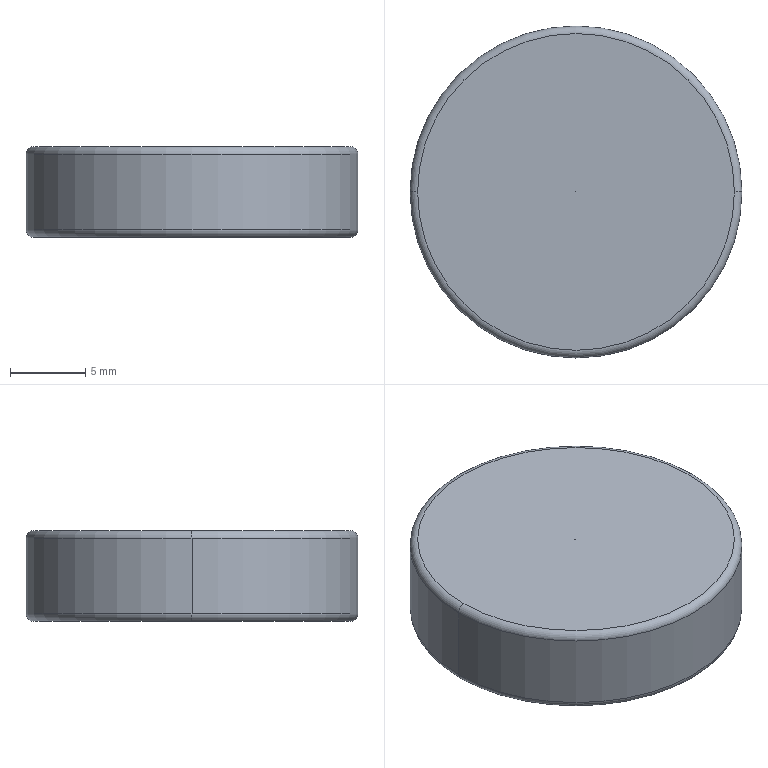Part | STEP file | H_ND24021-01-JG-036-SL | 1 solid | 12 faces | box 22 x 22 x 6 mm | volume 2228 mm3 | torus 4 | cylinder 4 | cone 2 | plane 2 | commonest cylinder face diameters 3.3 x2 22 x2
STEP:
#1=CARTESIAN_POINT('',(0.,0.,0.));
#2=DIRECTION('',(0.,0.,1.));
#3=DIRECTION('',(1.,0.,0.));
#4=AXIS2_PLACEMENT_3D('',#1,#2,#3);
#5=CARTESIAN_POINT('',(-11.,0.,5.5));
#6=VERTEX_POINT('',#5);
#7=CARTESIAN_POINT('',(11.,0.,5.5));
#8=VERTEX_POINT('',#7);
#9=CARTESIAN_POINT('',(0.,0.,5.5));
#10=DIRECTION('',(0.,0.,-1.));
#11=DIRECTION('',(1.,0.,0.));
#12=AXIS2_PLACEMENT_3D('',#9,#10,#11);
#13=CIRCLE('',#12,11.);
#14=CARTESIAN_POINT('',(0.,0.,5.5));
#15=DIRECTION('',(0.,0.,1.));
#16=DIRECTION('',(1.,0.,0.));
#17=AXIS2_PLACEMENT_3D('',#14,#15,#16);
#18=TOROIDAL_SURFACE('',#17,10.5,0.5);
#19=CARTESIAN_POINT('',(6.283,0.));
#20=DIRECTION('',(-1.,0.));
#21=VECTOR('',#20,1.);
#22=LINE('',#19,#21);
#23=(GEOMETRIC_REPRESENTATION_CONTEXT(2)PARAMETRIC_REPRESENTATION_CONTEXT()REPRESENTATION_CONTEXT('',''));
#24=DEFINITIONAL_REPRESENTATION('',(#22),#23);
#25=PCURVE('',#18,#24);
#26=CARTESIAN_POINT('',(0.,0.,6.));
#27=DIRECTION('',(0.,0.,-1.));
#28=DIRECTION('',(-1.,0.,0.));
#29=AXIS2_PLACEMENT_3D('',#26,#27,#28);
#30=CYLINDRICAL_SURFACE('',#29,11.);
#31=CARTESIAN_POINT('',(-3.142,0.5));
#32=DIRECTION('',(1.,0.));
#33=VECTOR('',#32,1.);
#34=LINE('',#31,#33);
#35=(GEOMETRIC_REPRESENTATION_CONTEXT(2)PARAMETRIC_REPRESENTATION_CONTEXT()REPRESENTATION_CONTEXT('',''));
#36=DEFINITIONAL_REPRESENTATION('',(#34),#35);
#37=PCURVE('',#30,#36);
#38=SURFACE_CURVE('',#13,(#25,#37),.PCURVE_S1.);
#39=EDGE_CURVE('',#6,#8,#38,.T.);
#40=ORIENTED_EDGE('',*,*,#39,.F.);
#41=CARTESIAN_POINT('',(-10.5,0.,6.));
#42=VERTEX_POINT('',#41);
#43=CARTESIAN_POINT('',(-10.5,0.,5.5));
#44=DIRECTION('',(0.,1.,0.));
#45=DIRECTION('',(-1.,0.,0.));
#46=AXIS2_PLACEMENT_3D('',#43,#44,#45);
#47=CIRCLE('',#46,0.5);
#48=CARTESIAN_POINT('',(3.142,0.));
#49=DIRECTION('',(0.,1.));
#50=VECTOR('',#49,1.);
#51=LINE('',#48,#50);
#52=(GEOMETRIC_REPRESENTATION_CONTEXT(2)PARAMETRIC_REPRESENTATION_CONTEXT()REPRESENTATION_CONTEXT('',''));
#53=DEFINITIONAL_REPRESENTATION('',(#51),#52);
#54=PCURVE('',#18,#53);
#55=CARTESIAN_POINT('',(0.,0.,5.5));
#56=DIRECTION('',(0.,0.,1.));
#57=DIRECTION('',(1.,0.,0.));
#58=AXIS2_PLACEMENT_3D('',#55,#56,#57);
#59=TOROIDAL_SURFACE('',#58,10.5,0.5);
#60=CARTESIAN_POINT('',(3.142,0.));
#61=DIRECTION('',(0.,1.));
#62=VECTOR('',#61,1.);
#63=LINE('',#60,#62);
#64=(GEOMETRIC_REPRESENTATION_CONTEXT(2)PARAMETRIC_REPRESENTATION_CONTEXT()REPRESENTATION_CONTEXT('',''));
#65=DEFINITIONAL_REPRESENTATION('',(#63),#64);
#66=PCURVE('',#59,#65);
#67=SURFACE_CURVE('',#47,(#54,#66),.PCURVE_S1.);
#68=EDGE_CURVE('',#6,#42,#67,.T.);
#69=ORIENTED_EDGE('',*,*,#68,.T.);
#70=CARTESIAN_POINT('',(10.5,0.,6.));
#71=VERTEX_POINT('',#70);
#72=CARTESIAN_POINT('',(0.,0.,6.));
#73=DIRECTION('',(0.,0.,1.));
#74=DIRECTION('',(1.,0.,0.));
#75=AXIS2_PLACEMENT_3D('',#72,#73,#74);
#76=CIRCLE('',#75,10.5);
#77=CARTESIAN_POINT('',(0.,1.571));
#78=DIRECTION('',(1.,0.));
#79=VECTOR('',#78,1.);
#80=LINE('',#77,#79);
#81=(GEOMETRIC_REPRESENTATION_CONTEXT(2)PARAMETRIC_REPRESENTATION_CONTEXT()REPRESENTATION_CONTEXT('',''));
#82=DEFINITIONAL_REPRESENTATION('',(#80),#81);
#83=PCURVE('',#18,#82);
#84=CARTESIAN_POINT('',(0.,0.,6.));
#85=DIRECTION('',(0.,0.,1.));
#86=DIRECTION('',(1.,0.,0.));
#87=AXIS2_PLACEMENT_3D('',#84,#85,#86);
#88=PLANE('',#87);
#89=CARTESIAN_POINT('',(0.,0.));
#90=DIRECTION('',(1.,0.));
#91=AXIS2_PLACEMENT_2D('',#89,#90);
#92=CIRCLE('',#91,10.5);
#93=(GEOMETRIC_REPRESENTATION_CONTEXT(2)PARAMETRIC_REPRESENTATION_CONTEXT()REPRESENTATION_CONTEXT('',''));
#94=DEFINITIONAL_REPRESENTATION('',(#92),#93);
#95=PCURVE('',#88,#94);
#96=SURFACE_CURVE('',#76,(#83,#95),.PCURVE_S1.);
#97=EDGE_CURVE('',#71,#42,#96,.T.);
#98=ORIENTED_EDGE('',*,*,#97,.F.);
#99=CARTESIAN_POINT('',(10.5,0.,5.5));
#100=DIRECTION('',(0.,-1.,0.));
#101=DIRECTION('',(0.,0.,-1.));
#102=AXIS2_PLACEMENT_3D('',#99,#100,#101);
#103=CIRCLE('',#102,0.5);
#104=CARTESIAN_POINT('',(0.,-1.571));
#105=DIRECTION('',(0.,1.));
#106=VECTOR('',#105,1.);
#107=LINE('',#104,#106);
#108=(GEOMETRIC_REPRESENTATION_CONTEXT(2)PARAMETRIC_REPRESENTATION_CONTEXT()REPRESENTATION_CONTEXT('',''));
#109=DEFINITIONAL_REPRESENTATION('',(#107),#108);
#110=PCURVE('',#18,#109);
#111=CARTESIAN_POINT('',(6.283,-1.571));
#112=DIRECTION('',(0.,1.));
#113=VECTOR('',#112,1.);
#114=LINE('',#111,#113);
#115=(GEOMETRIC_REPRESENTATION_CONTEXT(2)PARAMETRIC_REPRESENTATION_CONTEXT()REPRESENTATION_CONTEXT('',''));
#116=DEFINITIONAL_REPRESENTATION('',(#114),#115);
#117=PCURVE('',#59,#116);
#118=SURFACE_CURVE('',#103,(#110,#117),.PCURVE_S1.);
#119=EDGE_CURVE('',#8,#71,#118,.T.);
#120=ORIENTED_EDGE('',*,*,#119,.F.);
#121=EDGE_LOOP('',(#40,#69,#98,#120));
#122=FACE_BOUND('',#121,.T.);
#123=ADVANCED_FACE('',(#122),#18,.T.);
#124=CARTESIAN_POINT('',(-10.5,0.,0.));
#125=VERTEX_POINT('',#124);
#126=CARTESIAN_POINT('',(10.5,0.,0.));
#127=VERTEX_POINT('',#126);
#128=CARTESIAN_POINT('',(0.,0.,0.));
#129=DIRECTION('',(0.,0.,-1.));
#130=DIRECTION('',(1.,0.,0.));
#131=AXIS2_PLACEMENT_3D('',#128,#129,#130);
#132=CIRCLE('',#131,10.5);
#133=CARTESIAN_POINT('',(0.,0.,0.5));
#134=DIRECTION('',(0.,0.,1.));
#135=DIRECTION('',(1.,0.,0.));
#136=AXIS2_PLACEMENT_3D('',#133,#134,#135);
#137=TOROIDAL_SURFACE('',#136,10.5,0.5);
#138=CARTESIAN_POINT('',(6.283,4.712));
#139=DIRECTION('',(-1.,0.));
#140=VECTOR('',#139,1.);
#141=LINE('',#138,#140);
#142=(GEOMETRIC_REPRESENTATION_CONTEXT(2)PARAMETRIC_REPRESENTATION_CONTEXT()REPRESENTATION_CONTEXT('',''));
#143=DEFINITIONAL_REPRESENTATION('',(#141),#142);
#144=PCURVE('',#137,#143);
#145=CARTESIAN_POINT('',(0.,0.,0.));
#146=DIRECTION('',(0.,0.,1.));
#147=DIRECTION('',(1.,0.,0.));
#148=AXIS2_PLACEMENT_3D('',#145,#146,#147);
#149=PLANE('',#148);
#150=CARTESIAN_POINT('',(10.5,0.));
#151=CARTESIAN_POINT('',(10.5,-18.187));
#152=CARTESIAN_POINT('',(-5.25,-9.093));
#153=CARTESIAN_POINT('',(-21.,0.));
#154=CARTESIAN_POINT('',(-5.25,9.093));
#155=CARTESIAN_POINT('',(10.5,18.187));
#156=CARTESIAN_POINT('',(10.5,0.));
#157=(BOUNDED_CURVE()B_SPLINE_CURVE(2,(#150,#151,#152,#153,#154,#155,#156),.UNSPECIFIED.,.T.,.F.)B_SPLINE_CURVE_WITH_KNOTS((1,2,2,2,2,1),(-2.094,0.,2.094,4.189,6.283,8.378),.UNSPECIFIED.)CURVE()GEOMETRIC_REPRESENTATION_ITEM()RATIONAL_B_SPLINE_CURVE((1.,0.5,1.,0.5,1.,0.5,1.))REPRESENTATION_ITEM(''));
#158=(GEOMETRIC_REPRESENTATION_CONTEXT(2)PARAMETRIC_REPRESENTATION_CONTEXT()REPRESENTATION_CONTEXT('',''));
#159=DEFINITIONAL_REPRESENTATION('',(#157),#158);
#160=PCURVE('',#149,#159);
#161=SURFACE_CURVE('',#132,(#144,#160),.PCURVE_S1.);
#162=EDGE_CURVE('',#125,#127,#161,.T.);
#163=ORIENTED_EDGE('',*,*,#162,.F.);
#164=CARTESIAN_POINT('',(-11.,0.,0.5));
#165=VERTEX_POINT('',#164);
#166=CARTESIAN_POINT('',(-10.5,0.,0.5));
#167=DIRECTION('',(0.,1.,0.));
#168=DIRECTION('',(-1.,0.,0.));
#169=AXIS2_PLACEMENT_3D('',#166,#167,#168);
#170=CIRCLE('',#169,0.5);
#171=CARTESIAN_POINT('',(3.142,0.));
#172=DIRECTION('',(0.,1.));
#173=VECTOR('',#172,1.);
#174=LINE('',#171,#173);
#175=(GEOMETRIC_REPRESENTATION_CONTEXT(2)PARAMETRIC_REPRESENTATION_CONTEXT()REPRESENTATION_CONTEXT('',''));
#176=DEFINITIONAL_REPRESENTATION('',(#174),#175);
#177=PCURVE('',#137,#176);
#178=CARTESIAN_POINT('',(0.,0.,0.5));
#179=DIRECTION('',(0.,0.,1.));
#180=DIRECTION('',(1.,0.,0.));
#181=AXIS2_PLACEMENT_3D('',#178,#179,#180);
#182=TOROIDAL_SURFACE('',#181,10.5,0.5);
#183=CARTESIAN_POINT('',(3.142,0.));
#184=DIRECTION('',(0.,1.));
#185=VECTOR('',#184,1.);
#186=LINE('',#183,#185);
#187=(GEOMETRIC_REPRESENTATION_CONTEXT(2)PARAMETRIC_REPRESENTATION_CONTEXT()REPRESENTATION_CONTEXT('',''));
#188=DEFINITIONAL_REPRESENTATION('',(#186),#187);
#189=PCURVE('',#182,#188);
#190=SURFACE_CURVE('',#170,(#177,#189),.PCURVE_S1.);
#191=EDGE_CURVE('',#125,#165,#190,.T.);
#192=ORIENTED_EDGE('',*,*,#191,.T.);
#193=CARTESIAN_POINT('',(11.,0.,0.5));
#194=VERTEX_POINT('',#193);
#195=CARTESIAN_POINT('',(0.,0.,0.5));
#196=DIRECTION('',(0.,0.,1.));
#197=DIRECTION('',(1.,0.,0.));
#198=AXIS2_PLACEMENT_3D('',#195,#196,#197);
#199=CIRCLE('',#198,11.);
#200=CARTESIAN_POINT('',(0.,6.283));
#201=DIRECTION('',(1.,0.));
#202=VECTOR('',#201,1.);
#203=LINE('',#200,#202);
#204=(GEOMETRIC_REPRESENTATION_CONTEXT(2)PARAMETRIC_REPRESENTATION_CONTEXT()REPRESENTATION_CONTEXT('',''));
#205=DEFINITIONAL_REPRESENTATION('',(#203),#204);
#206=PCURVE('',#137,#205);
#207=CARTESIAN_POINT('',(3.142,5.5));
#208=DIRECTION('',(-1.,0.));
#209=VECTOR('',#208,1.);
#210=LINE('',#207,#209);
#211=(GEOMETRIC_REPRESENTATION_CONTEXT(2)PARAMETRIC_REPRESENTATION_CONTEXT()REPRESENTATION_CONTEXT('',''));
#212=DEFINITIONAL_REPRESENTATION('',(#210),#211);
#213=PCURVE('',#30,#212);
#214=SURFACE_CURVE('',#199,(#206,#213),.PCURVE_S1.);
#215=EDGE_CURVE('',#194,#165,#214,.T.);
#216=ORIENTED_EDGE('',*,*,#215,.F.);
#217=CARTESIAN_POINT('',(10.5,0.,0.5));
#218=DIRECTION('',(0.,-1.,0.));
#219=DIRECTION('',(0.,0.,-1.));
#220=AXIS2_PLACEMENT_3D('',#217,#218,#219);
#221=CIRCLE('',#220,0.5);
#222=CARTESIAN_POINT('',(0.,4.712));
#223=DIRECTION('',(0.,1.));
#224=VECTOR('',#223,1.);
#225=LINE('',#222,#224);
#226=(GEOMETRIC_REPRESENTATION_CONTEXT(2)PARAMETRIC_REPRESENTATION_CONTEXT()REPRESENTATION_CONTEXT('',''));
#227=DEFINITIONAL_REPRESENTATION('',(#225),#226);
#228=PCURVE('',#137,#227);
#229=CARTESIAN_POINT('',(6.283,4.712));
#230=DIRECTION('',(0.,1.));
#231=VECTOR('',#230,1.);
#232=LINE('',#229,#231);
#233=(GEOMETRIC_REPRESENTATION_CONTEXT(2)PARAMETRIC_REPRESENTATION_CONTEXT()REPRESENTATION_CONTEXT('',''));
#234=DEFINITIONAL_REPRESENTATION('',(#232),#233);
#235=PCURVE('',#182,#234);
#236=SURFACE_CURVE('',#221,(#228,#235),.PCURVE_S1.);
#237=EDGE_CURVE('',#127,#194,#236,.T.);
#238=ORIENTED_EDGE('',*,*,#237,.F.);
#239=EDGE_LOOP('',(#163,#192,#216,#238));
#240=FACE_BOUND('',#239,.T.);
#241=ADVANCED_FACE('',(#240),#137,.T.);
#242=CARTESIAN_POINT('',(-1.65,0.,5.));
#243=VERTEX_POINT('',#242);
#244=CARTESIAN_POINT('',(-1.65,0.,0.));
#245=VERTEX_POINT('',#244);
#246=CARTESIAN_POINT('',(-1.65,0.,0.));
#247=DIRECTION('',(0.,0.,-1.));
#248=VECTOR('',#247,1.);
#249=LINE('',#246,#248);
#250=CARTESIAN_POINT('',(0.,0.,0.));
#251=DIRECTION('',(0.,0.,-1.));
#252=DIRECTION('',(-1.,0.,0.));
#253=AXIS2_PLACEMENT_3D('',#250,#251,#252);
#254=CYLINDRICAL_SURFACE('',#253,1.65);
#255=CARTESIAN_POINT('',(6.283,0.));
#256=DIRECTION('',(0.,1.));
#257=VECTOR('',#256,1.);
#258=LINE('',#255,#257);
#259=(GEOMETRIC_REPRESENTATION_CONTEXT(2)PARAMETRIC_REPRESENTATION_CONTEXT()REPRESENTATION_CONTEXT('',''));
#260=DEFINITIONAL_REPRESENTATION('',(#258),#259);
#261=PCURVE('',#254,#260);
#262=CARTESIAN_POINT('',(0.,0.,0.));
#263=DIRECTION('',(0.,0.,-1.));
#264=DIRECTION('',(-1.,0.,0.));
#265=AXIS2_PLACEMENT_3D('',#262,#263,#264);
#266=CYLINDRICAL_SURFACE('',#265,1.65);
#267=CARTESIAN_POINT('',(0.,0.));
#268=DIRECTION('',(0.,1.));
#269=VECTOR('',#268,1.);
#270=LINE('',#267,#269);
#271=(GEOMETRIC_REPRESENTATION_CONTEXT(2)PARAMETRIC_REPRESENTATION_CONTEXT()REPRESENTATION_CONTEXT('',''));
#272=DEFINITIONAL_REPRESENTATION('',(#270),#271);
#273=PCURVE('',#266,#272);
#274=SURFACE_CURVE('',#249,(#261,#273),.PCURVE_S1.);
#275=EDGE_CURVE('',#243,#245,#274,.T.);
#276=ORIENTED_EDGE('',*,*,#275,.T.);
#277=CARTESIAN_POINT('',(1.65,0.,0.));
#278=VERTEX_POINT('',#277);
#279=CARTESIAN_POINT('',(0.,0.,0.));
#280=DIRECTION('',(0.,0.,-1.));
#281=DIRECTION('',(-1.,0.,0.));
#282=AXIS2_PLACEMENT_3D('',#279,#280,#281);
#283=CIRCLE('',#282,1.65);
#284=CARTESIAN_POINT('',(0.,0.));
#285=DIRECTION('',(1.,0.));
#286=VECTOR('',#285,1.);
#287=LINE('',#284,#286);
#288=(GEOMETRIC_REPRESENTATION_CONTEXT(2)PARAMETRIC_REPRESENTATION_CONTEXT()REPRESENTATION_CONTEXT('',''));
#289=DEFINITIONAL_REPRESENTATION('',(#287),#288);
#290=PCURVE('',#254,#289);
#291=CARTESIAN_POINT('',(-1.65,0.));
#292=CARTESIAN_POINT('',(-1.65,2.858));
#293=CARTESIAN_POINT('',(0.825,1.429));
#294=CARTESIAN_POINT('',(3.3,0.));
#295=CARTESIAN_POINT('',(0.825,-1.429));
#296=CARTESIAN_POINT('',(-1.65,-2.858));
#297=CARTESIAN_POINT('',(-1.65,0.));
#298=(BOUNDED_CURVE()B_SPLINE_CURVE(2,(#291,#292,#293,#294,#295,#296,#297),.UNSPECIFIED.,.T.,.F.)B_SPLINE_CURVE_WITH_KNOTS((1,2,2,2,2,1),(-2.094,0.,2.094,4.189,6.283,8.378),.UNSPECIFIED.)CURVE()GEOMETRIC_REPRESENTATION_ITEM()RATIONAL_B_SPLINE_CURVE((1.,0.5,1.,0.5,1.,0.5,1.))REPRESENTATION_ITEM(''));
#299=(GEOMETRIC_REPRESENTATION_CONTEXT(2)PARAMETRIC_REPRESENTATION_CONTEXT()REPRESENTATION_CONTEXT('',''));
#300=DEFINITIONAL_REPRESENTATION('',(#298),#299);
#301=PCURVE('',#149,#300);
#302=SURFACE_CURVE('',#283,(#290,#301),.PCURVE_S1.);
#303=EDGE_CURVE('',#278,#245,#302,.T.);
#304=ORIENTED_EDGE('',*,*,#303,.F.);
#305=CARTESIAN_POINT('',(1.65,0.,5.));
#306=VERTEX_POINT('',#305);
#307=CARTESIAN_POINT('',(1.65,0.,0.));
#308=DIRECTION('',(0.,0.,-1.));
#309=VECTOR('',#308,1.);
#310=LINE('',#307,#309);
#311=CARTESIAN_POINT('',(3.142,0.));
#312=DIRECTION('',(0.,1.));
#313=VECTOR('',#312,1.);
#314=LINE('',#311,#313);
#315=(GEOMETRIC_REPRESENTATION_CONTEXT(2)PARAMETRIC_REPRESENTATION_CONTEXT()REPRESENTATION_CONTEXT('',''));
#316=DEFINITIONAL_REPRESENTATION('',(#314),#315);
#317=PCURVE('',#254,#316);
#318=CARTESIAN_POINT('',(3.142,0.));
#319=DIRECTION('',(0.,1.));
#320=VECTOR('',#319,1.);
#321=LINE('',#318,#320);
#322=(GEOMETRIC_REPRESENTATION_CONTEXT(2)PARAMETRIC_REPRESENTATION_CONTEXT()REPRESENTATION_CONTEXT('',''));
#323=DEFINITIONAL_REPRESENTATION('',(#321),#322);
#324=PCURVE('',#266,#323);
#325=SURFACE_CURVE('',#310,(#317,#324),.PCURVE_S1.);
#326=EDGE_CURVE('',#306,#278,#325,.T.);
#327=ORIENTED_EDGE('',*,*,#326,.F.);
#328=CARTESIAN_POINT('',(0.,0.,5.));
#329=DIRECTION('',(0.,0.,-1.));
#330=DIRECTION('',(-1.,0.,0.));
#331=AXIS2_PLACEMENT_3D('',#328,#329,#330);
#332=CIRCLE('',#331,1.65);
#333=CARTESIAN_POINT('',(0.,-5.));
#334=DIRECTION('',(1.,0.));
#335=VECTOR('',#334,1.);
#336=LINE('',#333,#335);
#337=(GEOMETRIC_REPRESENTATION_CONTEXT(2)PARAMETRIC_REPRESENTATION_CONTEXT()REPRESENTATION_CONTEXT('',''));
#338=DEFINITIONAL_REPRESENTATION('',(#336),#337);
#339=PCURVE('',#254,#338);
#340=CARTESIAN_POINT('',(0.,0.,5.));
#341=DIRECTION('',(0.,0.,-1.));
#342=DIRECTION('',(-1.,0.,0.));
#343=AXIS2_PLACEMENT_3D('',#340,#341,#342);
#344=CONICAL_SURFACE('',#343,1.65,1.03);
#345=CARTESIAN_POINT('',(0.,0.));
#346=DIRECTION('',(1.,0.));
#347=VECTOR('',#346,1.);
#348=LINE('',#345,#347);
#349=(GEOMETRIC_REPRESENTATION_CONTEXT(2)PARAMETRIC_REPRESENTATION_CONTEXT()REPRESENTATION_CONTEXT('',''));
#350=DEFINITIONAL_REPRESENTATION('',(#348),#349);
#351=PCURVE('',#344,#350);
#352=SURFACE_CURVE('',#332,(#339,#351),.PCURVE_S1.);
#353=EDGE_CURVE('',#306,#243,#352,.T.);
#354=ORIENTED_EDGE('',*,*,#353,.T.);
#355=EDGE_LOOP('',(#276,#304,#327,#354));
#356=FACE_BOUND('',#355,.F.);
#357=ADVANCED_FACE('',(#356),#254,.F.);
#358=ORIENTED_EDGE('',*,*,#353,.F.);
#359=CARTESIAN_POINT('',(0.,0.,5.991));
#360=VERTEX_POINT('',#359);
#361=CARTESIAN_POINT('',(1.65,0.,5.));
#362=DIRECTION('',(0.8572,0.,-0.515));
#363=VECTOR('',#362,1.);
#364=LINE('',#361,#363);
#365=CARTESIAN_POINT('',(3.142,0.));
#366=DIRECTION('',(0.,1.));
#367=VECTOR('',#366,1.);
#368=LINE('',#365,#367);
#369=(GEOMETRIC_REPRESENTATION_CONTEXT(2)PARAMETRIC_REPRESENTATION_CONTEXT()REPRESENTATION_CONTEXT('',''));
#370=DEFINITIONAL_REPRESENTATION('',(#368),#369);
#371=PCURVE('',#344,#370);
#372=CARTESIAN_POINT('',(0.,0.,5.));
#373=DIRECTION('',(0.,0.,-1.));
#374=DIRECTION('',(-1.,0.,0.));
#375=AXIS2_PLACEMENT_3D('',#372,#373,#374);
#376=CONICAL_SURFACE('',#375,1.65,1.03);
#377=CARTESIAN_POINT('',(3.142,0.));
#378=DIRECTION('',(0.,1.));
#379=VECTOR('',#378,1.);
#380=LINE('',#377,#379);
#381=(GEOMETRIC_REPRESENTATION_CONTEXT(2)PARAMETRIC_REPRESENTATION_CONTEXT()REPRESENTATION_CONTEXT('',''));
#382=DEFINITIONAL_REPRESENTATION('',(#380),#381);
#383=PCURVE('',#376,#382);
#384=SURFACE_CURVE('',#364,(#371,#383),.PCURVE_S1.);
#385=EDGE_CURVE('',#360,#306,#384,.T.);
#386=ORIENTED_EDGE('',*,*,#385,.F.);
#387=CARTESIAN_POINT('',(-1.65,0.,5.));
#388=DIRECTION('',(-0.8572,0.,-0.515));
#389=VECTOR('',#388,1.);
#390=LINE('',#387,#389);
#391=CARTESIAN_POINT('',(6.283,0.));
#392=DIRECTION('',(0.,1.));
#393=VECTOR('',#392,1.);
#394=LINE('',#391,#393);
#395=(GEOMETRIC_REPRESENTATION_CONTEXT(2)PARAMETRIC_REPRESENTATION_CONTEXT()REPRESENTATION_CONTEXT('',''));
#396=DEFINITIONAL_REPRESENTATION('',(#394),#395);
#397=PCURVE('',#344,#396);
#398=CARTESIAN_POINT('',(0.,0.));
#399=DIRECTION('',(0.,1.));
#400=VECTOR('',#399,1.);
#401=LINE('',#398,#400);
#402=(GEOMETRIC_REPRESENTATION_CONTEXT(2)PARAMETRIC_REPRESENTATION_CONTEXT()REPRESENTATION_CONTEXT('',''));
#403=DEFINITIONAL_REPRESENTATION('',(#401),#402);
#404=PCURVE('',#376,#403);
#405=SURFACE_CURVE('',#390,(#397,#404),.PCURVE_S1.);
#406=EDGE_CURVE('',#360,#243,#405,.T.);
#407=ORIENTED_EDGE('',*,*,#406,.T.);
#408=EDGE_LOOP('',(#358,#386,#407));
#409=FACE_BOUND('',#408,.F.);
#410=ADVANCED_FACE('',(#409),#344,.F.);
#411=ORIENTED_EDGE('',*,*,#39,.T.);
#412=CARTESIAN_POINT('',(11.,0.,6.));
#413=DIRECTION('',(0.,0.,-1.));
#414=VECTOR('',#413,1.);
#415=LINE('',#412,#414);
#416=CARTESIAN_POINT('',(3.142,0.));
#417=DIRECTION('',(0.,1.));
#418=VECTOR('',#417,1.);
#419=LINE('',#416,#418);
#420=(GEOMETRIC_REPRESENTATION_CONTEXT(2)PARAMETRIC_REPRESENTATION_CONTEXT()REPRESENTATION_CONTEXT('',''));
#421=DEFINITIONAL_REPRESENTATION('',(#419),#420);
#422=PCURVE('',#30,#421);
#423=CARTESIAN_POINT('',(0.,0.,6.));
#424=DIRECTION('',(0.,0.,-1.));
#425=DIRECTION('',(-1.,0.,0.));
#426=AXIS2_PLACEMENT_3D('',#423,#424,#425);
#427=CYLINDRICAL_SURFACE('',#426,11.);
#428=CARTESIAN_POINT('',(3.142,0.));
#429=DIRECTION('',(0.,1.));
#430=VECTOR('',#429,1.);
#431=LINE('',#428,#430);
#432=(GEOMETRIC_REPRESENTATION_CONTEXT(2)PARAMETRIC_REPRESENTATION_CONTEXT()REPRESENTATION_CONTEXT('',''));
#433=DEFINITIONAL_REPRESENTATION('',(#431),#432);
#434=PCURVE('',#427,#433);
#435=SURFACE_CURVE('',#415,(#422,#434),.PCURVE_S1.);
#436=EDGE_CURVE('',#8,#194,#435,.T.);
#437=ORIENTED_EDGE('',*,*,#436,.T.);
#438=ORIENTED_EDGE('',*,*,#215,.T.);
#439=CARTESIAN_POINT('',(-11.,0.,6.));
#440=DIRECTION('',(0.,0.,-1.));
#441=VECTOR('',#440,1.);
#442=LINE('',#439,#441);
#443=CARTESIAN_POINT('',(0.,0.));
#444=DIRECTION('',(0.,1.));
#445=VECTOR('',#444,1.);
#446=LINE('',#443,#445);
#447=(GEOMETRIC_REPRESENTATION_CONTEXT(2)PARAMETRIC_REPRESENTATION_CONTEXT()REPRESENTATION_CONTEXT('',''));
#448=DEFINITIONAL_REPRESENTATION('',(#446),#447);
#449=PCURVE('',#30,#448);
#450=CARTESIAN_POINT('',(6.283,0.));
#451=DIRECTION('',(0.,1.));
#452=VECTOR('',#451,1.);
#453=LINE('',#450,#452);
#454=(GEOMETRIC_REPRESENTATION_CONTEXT(2)PARAMETRIC_REPRESENTATION_CONTEXT()REPRESENTATION_CONTEXT('',''));
#455=DEFINITIONAL_REPRESENTATION('',(#453),#454);
#456=PCURVE('',#427,#455);
#457=SURFACE_CURVE('',#442,(#449,#456),.PCURVE_S1.);
#458=EDGE_CURVE('',#6,#165,#457,.T.);
#459=ORIENTED_EDGE('',*,*,#458,.F.);
#460=EDGE_LOOP('',(#411,#437,#438,#459));
#461=FACE_BOUND('',#460,.T.);
#462=ADVANCED_FACE('',(#461),#30,.T.);
#463=ORIENTED_EDGE('',*,*,#436,.F.);
#464=CARTESIAN_POINT('',(0.,0.,5.5));
#465=DIRECTION('',(0.,0.,-1.));
#466=DIRECTION('',(1.,0.,0.));
#467=AXIS2_PLACEMENT_3D('',#464,#465,#466);
#468=CIRCLE('',#467,11.);
#469=CARTESIAN_POINT('',(3.142,0.5));
#470=DIRECTION('',(1.,0.));
#471=VECTOR('',#470,1.);
#472=LINE('',#469,#471);
#473=(GEOMETRIC_REPRESENTATION_CONTEXT(2)PARAMETRIC_REPRESENTATION_CONTEXT()REPRESENTATION_CONTEXT('',''));
#474=DEFINITIONAL_REPRESENTATION('',(#472),#473);
#475=PCURVE('',#427,#474);
#476=CARTESIAN_POINT('',(6.283,0.));
#477=DIRECTION('',(-1.,0.));
#478=VECTOR('',#477,1.);
#479=LINE('',#476,#478);
#480=(GEOMETRIC_REPRESENTATION_CONTEXT(2)PARAMETRIC_REPRESENTATION_CONTEXT()REPRESENTATION_CONTEXT('',''));
#481=DEFINITIONAL_REPRESENTATION('',(#479),#480);
#482=PCURVE('',#59,#481);
#483=SURFACE_CURVE('',#468,(#475,#482),.PCURVE_S1.);
#484=EDGE_CURVE('',#8,#6,#483,.T.);
#485=ORIENTED_EDGE('',*,*,#484,.T.);
#486=ORIENTED_EDGE('',*,*,#458,.T.);
#487=CARTESIAN_POINT('',(0.,0.,0.5));
#488=DIRECTION('',(0.,0.,1.));
#489=DIRECTION('',(1.,0.,0.));
#490=AXIS2_PLACEMENT_3D('',#487,#488,#489);
#491=CIRCLE('',#490,11.);
#492=CARTESIAN_POINT('',(9.425,5.5));
#493=DIRECTION('',(-1.,0.));
#494=VECTOR('',#493,1.);
#495=LINE('',#492,#494);
#496=(GEOMETRIC_REPRESENTATION_CONTEXT(2)PARAMETRIC_REPRESENTATION_CONTEXT()REPRESENTATION_CONTEXT('',''));
#497=DEFINITIONAL_REPRESENTATION('',(#495),#496);
#498=PCURVE('',#427,#497);
#499=CARTESIAN_POINT('',(0.,6.283));
#500=DIRECTION('',(1.,0.));
#501=VECTOR('',#500,1.);
#502=LINE('',#499,#501);
#503=(GEOMETRIC_REPRESENTATION_CONTEXT(2)PARAMETRIC_REPRESENTATION_CONTEXT()REPRESENTATION_CONTEXT('',''));
#504=DEFINITIONAL_REPRESENTATION('',(#502),#503);
#505=PCURVE('',#182,#504);
#506=SURFACE_CURVE('',#491,(#498,#505),.PCURVE_S1.);
#507=EDGE_CURVE('',#165,#194,#506,.T.);
#508=ORIENTED_EDGE('',*,*,#507,.T.);
#509=EDGE_LOOP('',(#463,#485,#486,#508));
#510=FACE_BOUND('',#509,.T.);
#511=ADVANCED_FACE('',(#510),#427,.T.);
#512=ORIENTED_EDGE('',*,*,#97,.T.);
#513=CARTESIAN_POINT('',(0.,0.,6.));
#514=DIRECTION('',(0.,0.,1.));
#515=DIRECTION('',(1.,0.,0.));
#516=AXIS2_PLACEMENT_3D('',#513,#514,#515);
#517=CIRCLE('',#516,10.5);
#518=CARTESIAN_POINT('',(0.,0.));
#519=DIRECTION('',(1.,0.));
#520=AXIS2_PLACEMENT_2D('',#518,#519);
#521=CIRCLE('',#520,10.5);
#522=(GEOMETRIC_REPRESENTATION_CONTEXT(2)PARAMETRIC_REPRESENTATION_CONTEXT()REPRESENTATION_CONTEXT('',''));
#523=DEFINITIONAL_REPRESENTATION('',(#521),#522);
#524=PCURVE('',#88,#523);
#525=CARTESIAN_POINT('',(0.,1.571));
#526=DIRECTION('',(1.,0.));
#527=VECTOR('',#526,1.);
#528=LINE('',#525,#527);
#529=(GEOMETRIC_REPRESENTATION_CONTEXT(2)PARAMETRIC_REPRESENTATION_CONTEXT()REPRESENTATION_CONTEXT('',''));
#530=DEFINITIONAL_REPRESENTATION('',(#528),#529);
#531=PCURVE('',#59,#530);
#532=SURFACE_CURVE('',#517,(#524,#531),.PCURVE_S1.);
#533=EDGE_CURVE('',#42,#71,#532,.T.);
#534=ORIENTED_EDGE('',*,*,#533,.T.);
#535=EDGE_LOOP('',(#512,#534));
#536=FACE_BOUND('',#535,.T.);
#537=ADVANCED_FACE('',(#536),#88,.T.);
#538=CARTESIAN_POINT('',(0.,0.,0.));
#539=DIRECTION('',(0.,0.,-1.));
#540=DIRECTION('',(1.,0.,0.));
#541=AXIS2_PLACEMENT_3D('',#538,#539,#540);
#542=CIRCLE('',#541,10.5);
#543=CARTESIAN_POINT('',(10.5,0.));
#544=CARTESIAN_POINT('',(10.5,-18.187));
#545=CARTESIAN_POINT('',(-5.25,-9.093));
#546=CARTESIAN_POINT('',(-21.,0.));
#547=CARTESIAN_POINT('',(-5.25,9.093));
#548=CARTESIAN_POINT('',(10.5,18.187));
#549=CARTESIAN_POINT('',(10.5,0.));
#550=(BOUNDED_CURVE()B_SPLINE_CURVE(2,(#543,#544,#545,#546,#547,#548,#549),.UNSPECIFIED.,.T.,.F.)B_SPLINE_CURVE_WITH_KNOTS((1,2,2,2,2,1),(-2.094,0.,2.094,4.189,6.283,8.378),.UNSPECIFIED.)CURVE()GEOMETRIC_REPRESENTATION_ITEM()RATIONAL_B_SPLINE_CURVE((1.,0.5,1.,0.5,1.,0.5,1.))REPRESENTATION_ITEM(''));
#551=(GEOMETRIC_REPRESENTATION_CONTEXT(2)PARAMETRIC_REPRESENTATION_CONTEXT()REPRESENTATION_CONTEXT('',''));
#552=DEFINITIONAL_REPRESENTATION('',(#550),#551);
#553=PCURVE('',#149,#552);
#554=CARTESIAN_POINT('',(6.283,4.712));
#555=DIRECTION('',(-1.,0.));
#556=VECTOR('',#555,1.);
#557=LINE('',#554,#556);
#558=(GEOMETRIC_REPRESENTATION_CONTEXT(2)PARAMETRIC_REPRESENTATION_CONTEXT()REPRESENTATION_CONTEXT('',''));
#559=DEFINITIONAL_REPRESENTATION('',(#557),#558);
#560=PCURVE('',#182,#559);
#561=SURFACE_CURVE('',#542,(#553,#560),.PCURVE_S1.);
#562=EDGE_CURVE('',#127,#125,#561,.T.);
#563=ORIENTED_EDGE('',*,*,#562,.T.);
#564=ORIENTED_EDGE('',*,*,#162,.T.);
#565=EDGE_LOOP('',(#563,#564));
#566=FACE_BOUND('',#565,.T.);
#567=CARTESIAN_POINT('',(0.,0.,0.));
#568=DIRECTION('',(0.,0.,-1.));
#569=DIRECTION('',(-1.,0.,0.));
#570=AXIS2_PLACEMENT_3D('',#567,#568,#569);
#571=CIRCLE('',#570,1.65);
#572=CARTESIAN_POINT('',(-1.65,0.));
#573=CARTESIAN_POINT('',(-1.65,2.858));
#574=CARTESIAN_POINT('',(0.825,1.429));
#575=CARTESIAN_POINT('',(3.3,0.));
#576=CARTESIAN_POINT('',(0.825,-1.429));
#577=CARTESIAN_POINT('',(-1.65,-2.858));
#578=CARTESIAN_POINT('',(-1.65,0.));
#579=(BOUNDED_CURVE()B_SPLINE_CURVE(2,(#572,#573,#574,#575,#576,#577,#578),.UNSPECIFIED.,.T.,.F.)B_SPLINE_CURVE_WITH_KNOTS((1,2,2,2,2,1),(-2.094,0.,2.094,4.189,6.283,8.378),.UNSPECIFIED.)CURVE()GEOMETRIC_REPRESENTATION_ITEM()RATIONAL_B_SPLINE_CURVE((1.,0.5,1.,0.5,1.,0.5,1.))REPRESENTATION_ITEM(''));
#580=(GEOMETRIC_REPRESENTATION_CONTEXT(2)PARAMETRIC_REPRESENTATION_CONTEXT()REPRESENTATION_CONTEXT('',''));
#581=DEFINITIONAL_REPRESENTATION('',(#579),#580);
#582=PCURVE('',#149,#581);
#583=CARTESIAN_POINT('',(0.,0.));
#584=DIRECTION('',(1.,0.));
#585=VECTOR('',#584,1.);
#586=LINE('',#583,#585);
#587=(GEOMETRIC_REPRESENTATION_CONTEXT(2)PARAMETRIC_REPRESENTATION_CONTEXT()REPRESENTATION_CONTEXT('',''));
#588=DEFINITIONAL_REPRESENTATION('',(#586),#587);
#589=PCURVE('',#266,#588);
#590=SURFACE_CURVE('',#571,(#582,#589),.PCURVE_S1.);
#591=EDGE_CURVE('',#245,#278,#590,.T.);
#592=ORIENTED_EDGE('',*,*,#591,.F.);
#593=ORIENTED_EDGE('',*,*,#303,.F.);
#594=EDGE_LOOP('',(#592,#593));
#595=FACE_BOUND('',#594,.T.);
#596=ADVANCED_FACE('',(#566,#595),#149,.F.);
#597=CARTESIAN_POINT('',(0.,0.,5.));
#598=DIRECTION('',(0.,0.,-1.));
#599=DIRECTION('',(-1.,0.,0.));
#600=AXIS2_PLACEMENT_3D('',#597,#598,#599);
#601=CIRCLE('',#600,1.65);
#602=CARTESIAN_POINT('',(0.,0.));
#603=DIRECTION('',(1.,0.));
#604=VECTOR('',#603,1.);
#605=LINE('',#602,#604);
#606=(GEOMETRIC_REPRESENTATION_CONTEXT(2)PARAMETRIC_REPRESENTATION_CONTEXT()REPRESENTATION_CONTEXT('',''));
#607=DEFINITIONAL_REPRESENTATION('',(#605),#606);
#608=PCURVE('',#376,#607);
#609=CARTESIAN_POINT('',(0.,-5.));
#610=DIRECTION('',(1.,0.));
#611=VECTOR('',#610,1.);
#612=LINE('',#609,#611);
#613=(GEOMETRIC_REPRESENTATION_CONTEXT(2)PARAMETRIC_REPRESENTATION_CONTEXT()REPRESENTATION_CONTEXT('',''));
#614=DEFINITIONAL_REPRESENTATION('',(#612),#613);
#615=PCURVE('',#266,#614);
#616=SURFACE_CURVE('',#601,(#608,#615),.PCURVE_S1.);
#617=EDGE_CURVE('',#243,#306,#616,.T.);
#618=ORIENTED_EDGE('',*,*,#617,.F.);
#619=ORIENTED_EDGE('',*,*,#406,.F.);
#620=ORIENTED_EDGE('',*,*,#385,.T.);
#621=EDGE_LOOP('',(#618,#619,#620));
#622=FACE_BOUND('',#621,.F.);
#623=ADVANCED_FACE('',(#622),#376,.F.);
#624=ORIENTED_EDGE('',*,*,#591,.F.);
#625=ORIENTED_EDGE('',*,*,#275,.F.);
#626=ORIENTED_EDGE('',*,*,#617,.T.);
#627=ORIENTED_EDGE('',*,*,#326,.T.);
#628=EDGE_LOOP('',(#624,#625,#626,#627));
#629=FACE_BOUND('',#628,.F.);
#630=ADVANCED_FACE('',(#629),#266,.F.);
#631=ORIENTED_EDGE('',*,*,#191,.F.);
#632=ORIENTED_EDGE('',*,*,#562,.F.);
#633=ORIENTED_EDGE('',*,*,#237,.T.);
#634=ORIENTED_EDGE('',*,*,#507,.F.);
#635=EDGE_LOOP('',(#631,#632,#633,#634));
#636=FACE_BOUND('',#635,.T.);
#637=ADVANCED_FACE('',(#636),#182,.T.);
#638=ORIENTED_EDGE('',*,*,#68,.F.);
#639=ORIENTED_EDGE('',*,*,#484,.F.);
#640=ORIENTED_EDGE('',*,*,#119,.T.);
#641=ORIENTED_EDGE('',*,*,#533,.F.);
#642=EDGE_LOOP('',(#638,#639,#640,#641));
#643=FACE_BOUND('',#642,.T.);
#644=ADVANCED_FACE('',(#643),#59,.T.);
#645=CLOSED_SHELL('',(#123,#241,#357,#410,#462,#511,#537,#596,#623,#630,#637,#644));
#646=MANIFOLD_SOLID_BREP('',#645);
#647=(LENGTH_UNIT()NAMED_UNIT(*)SI_UNIT(.MILLI.,.METRE.));
#648=UNCERTAINTY_MEASURE_WITH_UNIT(LENGTH_MEASURE(0.0000001),#647,'','');
#649=(NAMED_UNIT(*)PLANE_ANGLE_UNIT()SI_UNIT($,.RADIAN.));
#650=(NAMED_UNIT(*)SI_UNIT($,.STERADIAN.)SOLID_ANGLE_UNIT());
#651=(GEOMETRIC_REPRESENTATION_CONTEXT(3)GLOBAL_UNCERTAINTY_ASSIGNED_CONTEXT((#648))GLOBAL_UNIT_ASSIGNED_CONTEXT((#647,#649,#650))REPRESENTATION_CONTEXT('',''));
#652=ADVANCED_BREP_SHAPE_REPRESENTATION('',(#4,#646),#651);